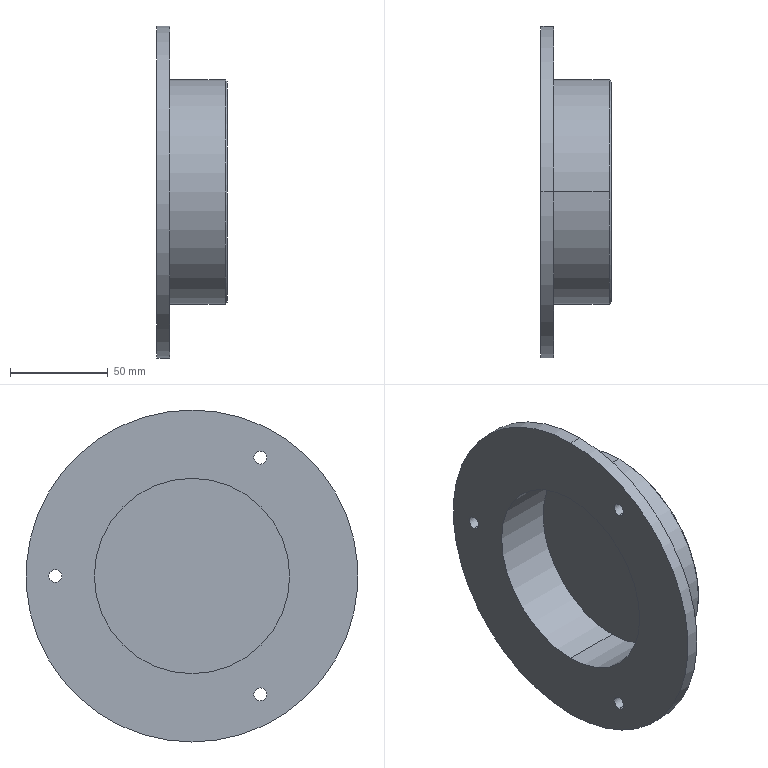Part | SolidWorks | features Chamfer 1, HoleWzd 1, Revolution 1 | 1 solid | 18 faces | box 36 x 170 x 170 mm | volume 217484 mm3 | cylinder 12 | plane 4 | cone 2 | commonest cylinder face diameters 6.6 x6 100 x2 115 x2 170 x2
STEP:
#1=CARTESIAN_POINT('',(36.,0.,-56.5));
#2=VERTEX_POINT('',#1);
#3=CARTESIAN_POINT('',(36.,0.,56.5));
#4=VERTEX_POINT('',#3);
#5=CARTESIAN_POINT('',(36.,0.,0.));
#6=DIRECTION('',(1.,0.,0.));
#7=DIRECTION('',(0.,0.,1.));
#8=AXIS2_PLACEMENT_3D('',#5,#6,#7);
#9=CIRCLE('',#8,56.5);
#10=EDGE_CURVE('',#2,#4,#9,.T.);
#11=ORIENTED_EDGE('',*,*,#10,.F.);
#12=CARTESIAN_POINT('',(35.,0.,-57.5));
#13=VERTEX_POINT('',#12);
#14=CARTESIAN_POINT('',(35.,0.,-57.5));
#15=DIRECTION('',(-0.7071,0.,-0.7071));
#16=VECTOR('',#15,1000.);
#17=LINE('',#14,#16);
#18=EDGE_CURVE('',#2,#13,#17,.T.);
#19=ORIENTED_EDGE('',*,*,#18,.T.);
#20=CARTESIAN_POINT('',(35.,0.,57.5));
#21=VERTEX_POINT('',#20);
#22=CARTESIAN_POINT('',(35.,0.,0.));
#23=DIRECTION('',(-1.,0.,0.));
#24=DIRECTION('',(0.,0.,1.));
#25=AXIS2_PLACEMENT_3D('',#22,#23,#24);
#26=CIRCLE('',#25,57.5);
#27=EDGE_CURVE('',#21,#13,#26,.T.);
#28=ORIENTED_EDGE('',*,*,#27,.F.);
#29=CARTESIAN_POINT('',(35.,0.,57.5));
#30=DIRECTION('',(-0.7071,0.,0.7071));
#31=VECTOR('',#30,1000.);
#32=LINE('',#29,#31);
#33=EDGE_CURVE('',#4,#21,#32,.T.);
#34=ORIENTED_EDGE('',*,*,#33,.F.);
#35=EDGE_LOOP('',(#11,#19,#28,#34));
#36=FACE_OUTER_BOUND('',#35,.T.);
#37=CARTESIAN_POINT('',(35.,0.,0.));
#38=DIRECTION('',(-1.,0.,0.));
#39=DIRECTION('',(0.,0.,1.));
#40=AXIS2_PLACEMENT_3D('',#37,#38,#39);
#41=CONICAL_SURFACE('',#40,57.5,0.7854);
#42=ADVANCED_FACE('',(#36),#41,.T.);
#43=CARTESIAN_POINT('',(0.,70.,3.3));
#44=VERTEX_POINT('',#43);
#45=CARTESIAN_POINT('',(0.,70.,-3.3));
#46=VERTEX_POINT('',#45);
#47=CARTESIAN_POINT('',(0.,70.,0.));
#48=DIRECTION('',(1.,0.,0.));
#49=DIRECTION('',(0.,0.,-1.));
#50=AXIS2_PLACEMENT_3D('',#47,#48,#49);
#51=CIRCLE('',#50,3.3);
#52=EDGE_CURVE('',#44,#46,#51,.T.);
#53=ORIENTED_EDGE('',*,*,#52,.F.);
#54=CARTESIAN_POINT('',(6.5,70.,3.3));
#55=VERTEX_POINT('',#54);
#56=CARTESIAN_POINT('',(6.5,70.,3.3));
#57=DIRECTION('',(1.,0.,0.));
#58=VECTOR('',#57,1000.);
#59=LINE('',#56,#58);
#60=EDGE_CURVE('',#44,#55,#59,.T.);
#61=ORIENTED_EDGE('',*,*,#60,.T.);
#62=CARTESIAN_POINT('',(6.5,70.,-3.3));
#63=VERTEX_POINT('',#62);
#64=CARTESIAN_POINT('',(6.5,70.,0.));
#65=DIRECTION('',(1.,0.,0.));
#66=DIRECTION('',(0.,0.,-1.));
#67=AXIS2_PLACEMENT_3D('',#64,#65,#66);
#68=CIRCLE('',#67,3.3);
#69=EDGE_CURVE('',#55,#63,#68,.T.);
#70=ORIENTED_EDGE('',*,*,#69,.T.);
#71=CARTESIAN_POINT('',(6.5,70.,-3.3));
#72=DIRECTION('',(1.,0.,0.));
#73=VECTOR('',#72,1000.);
#74=LINE('',#71,#73);
#75=EDGE_CURVE('',#46,#63,#74,.T.);
#76=ORIENTED_EDGE('',*,*,#75,.F.);
#77=EDGE_LOOP('',(#53,#61,#70,#76));
#78=FACE_OUTER_BOUND('',#77,.T.);
#79=CARTESIAN_POINT('',(6.5,70.,0.));
#80=DIRECTION('',(1.,0.,0.));
#81=DIRECTION('',(0.,0.,-1.));
#82=AXIS2_PLACEMENT_3D('',#79,#80,#81);
#83=CYLINDRICAL_SURFACE('',#82,3.3);
#84=ADVANCED_FACE('',(#78),#83,.F.);
#85=CARTESIAN_POINT('',(0.,-35.,-57.322));
#86=VERTEX_POINT('',#85);
#87=CARTESIAN_POINT('',(0.,-35.,-63.922));
#88=VERTEX_POINT('',#87);
#89=CARTESIAN_POINT('',(0.,-35.,-60.622));
#90=DIRECTION('',(1.,0.,0.));
#91=DIRECTION('',(0.,0.,-1.));
#92=AXIS2_PLACEMENT_3D('',#89,#90,#91);
#93=CIRCLE('',#92,3.3);
#94=EDGE_CURVE('',#86,#88,#93,.T.);
#95=ORIENTED_EDGE('',*,*,#94,.F.);
#96=CARTESIAN_POINT('',(6.5,-35.,-57.322));
#97=VERTEX_POINT('',#96);
#98=CARTESIAN_POINT('',(6.5,-35.,-57.322));
#99=DIRECTION('',(1.,0.,0.));
#100=VECTOR('',#99,1000.);
#101=LINE('',#98,#100);
#102=EDGE_CURVE('',#86,#97,#101,.T.);
#103=ORIENTED_EDGE('',*,*,#102,.T.);
#104=CARTESIAN_POINT('',(6.5,-35.,-63.922));
#105=VERTEX_POINT('',#104);
#106=CARTESIAN_POINT('',(6.5,-35.,-60.622));
#107=DIRECTION('',(1.,0.,0.));
#108=DIRECTION('',(0.,0.,-1.));
#109=AXIS2_PLACEMENT_3D('',#106,#107,#108);
#110=CIRCLE('',#109,3.3);
#111=EDGE_CURVE('',#97,#105,#110,.T.);
#112=ORIENTED_EDGE('',*,*,#111,.T.);
#113=CARTESIAN_POINT('',(6.5,-35.,-63.922));
#114=DIRECTION('',(1.,0.,0.));
#115=VECTOR('',#114,1000.);
#116=LINE('',#113,#115);
#117=EDGE_CURVE('',#88,#105,#116,.T.);
#118=ORIENTED_EDGE('',*,*,#117,.F.);
#119=EDGE_LOOP('',(#95,#103,#112,#118));
#120=FACE_OUTER_BOUND('',#119,.T.);
#121=CARTESIAN_POINT('',(6.5,-35.,-60.622));
#122=DIRECTION('',(1.,0.,0.));
#123=DIRECTION('',(0.,0.,-1.));
#124=AXIS2_PLACEMENT_3D('',#121,#122,#123);
#125=CYLINDRICAL_SURFACE('',#124,3.3);
#126=ADVANCED_FACE('',(#120),#125,.F.);
#127=CARTESIAN_POINT('',(0.,-35.,63.922));
#128=VERTEX_POINT('',#127);
#129=CARTESIAN_POINT('',(0.,-35.,57.322));
#130=VERTEX_POINT('',#129);
#131=CARTESIAN_POINT('',(0.,-35.,60.622));
#132=DIRECTION('',(1.,0.,0.));
#133=DIRECTION('',(0.,0.,-1.));
#134=AXIS2_PLACEMENT_3D('',#131,#132,#133);
#135=CIRCLE('',#134,3.3);
#136=EDGE_CURVE('',#128,#130,#135,.T.);
#137=ORIENTED_EDGE('',*,*,#136,.F.);
#138=CARTESIAN_POINT('',(6.5,-35.,63.922));
#139=VERTEX_POINT('',#138);
#140=CARTESIAN_POINT('',(6.5,-35.,63.922));
#141=DIRECTION('',(1.,0.,0.));
#142=VECTOR('',#141,1000.);
#143=LINE('',#140,#142);
#144=EDGE_CURVE('',#128,#139,#143,.T.);
#145=ORIENTED_EDGE('',*,*,#144,.T.);
#146=CARTESIAN_POINT('',(6.5,-35.,57.322));
#147=VERTEX_POINT('',#146);
#148=CARTESIAN_POINT('',(6.5,-35.,60.622));
#149=DIRECTION('',(1.,0.,0.));
#150=DIRECTION('',(0.,0.,-1.));
#151=AXIS2_PLACEMENT_3D('',#148,#149,#150);
#152=CIRCLE('',#151,3.3);
#153=EDGE_CURVE('',#139,#147,#152,.T.);
#154=ORIENTED_EDGE('',*,*,#153,.T.);
#155=CARTESIAN_POINT('',(6.5,-35.,57.322));
#156=DIRECTION('',(1.,0.,0.));
#157=VECTOR('',#156,1000.);
#158=LINE('',#155,#157);
#159=EDGE_CURVE('',#130,#147,#158,.T.);
#160=ORIENTED_EDGE('',*,*,#159,.F.);
#161=EDGE_LOOP('',(#137,#145,#154,#160));
#162=FACE_OUTER_BOUND('',#161,.T.);
#163=CARTESIAN_POINT('',(6.5,-35.,60.622));
#164=DIRECTION('',(1.,0.,0.));
#165=DIRECTION('',(0.,0.,-1.));
#166=AXIS2_PLACEMENT_3D('',#163,#164,#165);
#167=CYLINDRICAL_SURFACE('',#166,3.3);
#168=ADVANCED_FACE('',(#162),#167,.F.);
#169=ORIENTED_EDGE('',*,*,#27,.T.);
#170=CARTESIAN_POINT('',(6.5,0.,-57.5));
#171=VERTEX_POINT('',#170);
#172=CARTESIAN_POINT('',(0.,0.,-57.5));
#173=DIRECTION('',(-1.,0.,0.));
#174=VECTOR('',#173,1000.);
#175=LINE('',#172,#174);
#176=EDGE_CURVE('',#13,#171,#175,.T.);
#177=ORIENTED_EDGE('',*,*,#176,.T.);
#178=CARTESIAN_POINT('',(6.5,0.,57.5));
#179=VERTEX_POINT('',#178);
#180=CARTESIAN_POINT('',(6.5,0.,0.));
#181=DIRECTION('',(-1.,0.,0.));
#182=DIRECTION('',(0.,0.,1.));
#183=AXIS2_PLACEMENT_3D('',#180,#181,#182);
#184=CIRCLE('',#183,57.5);
#185=EDGE_CURVE('',#179,#171,#184,.T.);
#186=ORIENTED_EDGE('',*,*,#185,.F.);
#187=CARTESIAN_POINT('',(0.,0.,57.5));
#188=DIRECTION('',(-1.,0.,0.));
#189=VECTOR('',#188,1000.);
#190=LINE('',#187,#189);
#191=EDGE_CURVE('',#21,#179,#190,.T.);
#192=ORIENTED_EDGE('',*,*,#191,.F.);
#193=EDGE_LOOP('',(#169,#177,#186,#192));
#194=FACE_OUTER_BOUND('',#193,.T.);
#195=CARTESIAN_POINT('',(0.,0.,0.));
#196=DIRECTION('',(-1.,0.,0.));
#197=DIRECTION('',(0.,0.,1.));
#198=AXIS2_PLACEMENT_3D('',#195,#196,#197);
#199=CYLINDRICAL_SURFACE('',#198,57.5);
#200=ADVANCED_FACE('',(#194),#199,.T.);
#201=CARTESIAN_POINT('',(6.5,0.,85.));
#202=VERTEX_POINT('',#201);
#203=CARTESIAN_POINT('',(6.5,0.,-85.));
#204=VERTEX_POINT('',#203);
#205=CARTESIAN_POINT('',(6.5,0.,0.));
#206=DIRECTION('',(-1.,0.,0.));
#207=DIRECTION('',(0.,0.,1.));
#208=AXIS2_PLACEMENT_3D('',#205,#206,#207);
#209=CIRCLE('',#208,85.);
#210=EDGE_CURVE('',#202,#204,#209,.T.);
#211=ORIENTED_EDGE('',*,*,#210,.T.);
#212=CARTESIAN_POINT('',(0.,0.,-85.));
#213=VERTEX_POINT('',#212);
#214=CARTESIAN_POINT('',(0.,0.,-85.));
#215=DIRECTION('',(-1.,0.,0.));
#216=VECTOR('',#215,1000.);
#217=LINE('',#214,#216);
#218=EDGE_CURVE('',#204,#213,#217,.T.);
#219=ORIENTED_EDGE('',*,*,#218,.T.);
#220=CARTESIAN_POINT('',(0.,0.,85.));
#221=VERTEX_POINT('',#220);
#222=CARTESIAN_POINT('',(0.,0.,0.));
#223=DIRECTION('',(-1.,0.,0.));
#224=DIRECTION('',(0.,0.,1.));
#225=AXIS2_PLACEMENT_3D('',#222,#223,#224);
#226=CIRCLE('',#225,85.);
#227=EDGE_CURVE('',#221,#213,#226,.T.);
#228=ORIENTED_EDGE('',*,*,#227,.F.);
#229=CARTESIAN_POINT('',(0.,0.,85.));
#230=DIRECTION('',(-1.,0.,0.));
#231=VECTOR('',#230,1000.);
#232=LINE('',#229,#231);
#233=EDGE_CURVE('',#202,#221,#232,.T.);
#234=ORIENTED_EDGE('',*,*,#233,.F.);
#235=EDGE_LOOP('',(#211,#219,#228,#234));
#236=FACE_OUTER_BOUND('',#235,.T.);
#237=CARTESIAN_POINT('',(0.,0.,0.));
#238=DIRECTION('',(-1.,0.,0.));
#239=DIRECTION('',(0.,0.,1.));
#240=AXIS2_PLACEMENT_3D('',#237,#238,#239);
#241=CYLINDRICAL_SURFACE('',#240,85.);
#242=ADVANCED_FACE('',(#236),#241,.T.);
#243=CARTESIAN_POINT('',(30.,0.,-50.));
#244=VERTEX_POINT('',#243);
#245=CARTESIAN_POINT('',(30.,0.,50.));
#246=VERTEX_POINT('',#245);
#247=CARTESIAN_POINT('',(30.,0.,0.));
#248=DIRECTION('',(-1.,0.,0.));
#249=DIRECTION('',(0.,0.,1.));
#250=AXIS2_PLACEMENT_3D('',#247,#248,#249);
#251=CIRCLE('',#250,50.);
#252=EDGE_CURVE('',#244,#246,#251,.T.);
#253=ORIENTED_EDGE('',*,*,#252,.F.);
#254=CARTESIAN_POINT('',(0.,0.,-50.));
#255=VERTEX_POINT('',#254);
#256=CARTESIAN_POINT('',(0.,0.,-50.));
#257=DIRECTION('',(-1.,0.,0.));
#258=VECTOR('',#257,1000.);
#259=LINE('',#256,#258);
#260=EDGE_CURVE('',#244,#255,#259,.T.);
#261=ORIENTED_EDGE('',*,*,#260,.T.);
#262=CARTESIAN_POINT('',(0.,0.,50.));
#263=VERTEX_POINT('',#262);
#264=CARTESIAN_POINT('',(0.,0.,0.));
#265=DIRECTION('',(-1.,0.,0.));
#266=DIRECTION('',(0.,0.,1.));
#267=AXIS2_PLACEMENT_3D('',#264,#265,#266);
#268=CIRCLE('',#267,50.);
#269=EDGE_CURVE('',#255,#263,#268,.T.);
#270=ORIENTED_EDGE('',*,*,#269,.T.);
#271=CARTESIAN_POINT('',(0.,0.,50.));
#272=DIRECTION('',(-1.,0.,0.));
#273=VECTOR('',#272,1000.);
#274=LINE('',#271,#273);
#275=EDGE_CURVE('',#246,#263,#274,.T.);
#276=ORIENTED_EDGE('',*,*,#275,.F.);
#277=EDGE_LOOP('',(#253,#261,#270,#276));
#278=FACE_OUTER_BOUND('',#277,.T.);
#279=CARTESIAN_POINT('',(0.,0.,0.));
#280=DIRECTION('',(-1.,0.,0.));
#281=DIRECTION('',(0.,0.,1.));
#282=AXIS2_PLACEMENT_3D('',#279,#280,#281);
#283=CYLINDRICAL_SURFACE('',#282,50.);
#284=ADVANCED_FACE('',(#278),#283,.F.);
#285=CARTESIAN_POINT('',(6.5,70.,0.));
#286=DIRECTION('',(1.,0.,0.));
#287=DIRECTION('',(0.,0.,-1.));
#288=AXIS2_PLACEMENT_3D('',#285,#286,#287);
#289=CIRCLE('',#288,3.3);
#290=EDGE_CURVE('',#63,#55,#289,.T.);
#291=ORIENTED_EDGE('',*,*,#290,.F.);
#292=ORIENTED_EDGE('',*,*,#69,.F.);
#293=EDGE_LOOP('',(#291,#292));
#294=FACE_BOUND('',#293,.T.);
#295=ORIENTED_EDGE('',*,*,#210,.F.);
#296=CARTESIAN_POINT('',(6.5,0.,0.));
#297=DIRECTION('',(-1.,0.,0.));
#298=DIRECTION('',(0.,0.,1.));
#299=AXIS2_PLACEMENT_3D('',#296,#297,#298);
#300=CIRCLE('',#299,85.);
#301=EDGE_CURVE('',#204,#202,#300,.T.);
#302=ORIENTED_EDGE('',*,*,#301,.F.);
#303=EDGE_LOOP('',(#295,#302));
#304=FACE_OUTER_BOUND('',#303,.T.);
#305=ORIENTED_EDGE('',*,*,#185,.T.);
#306=CARTESIAN_POINT('',(6.5,0.,0.));
#307=DIRECTION('',(-1.,0.,0.));
#308=DIRECTION('',(0.,0.,1.));
#309=AXIS2_PLACEMENT_3D('',#306,#307,#308);
#310=CIRCLE('',#309,57.5);
#311=EDGE_CURVE('',#171,#179,#310,.T.);
#312=ORIENTED_EDGE('',*,*,#311,.T.);
#313=EDGE_LOOP('',(#305,#312));
#314=FACE_BOUND('',#313,.T.);
#315=CARTESIAN_POINT('',(6.5,-35.,60.622));
#316=DIRECTION('',(1.,0.,0.));
#317=DIRECTION('',(0.,0.,-1.));
#318=AXIS2_PLACEMENT_3D('',#315,#316,#317);
#319=CIRCLE('',#318,3.3);
#320=EDGE_CURVE('',#147,#139,#319,.T.);
#321=ORIENTED_EDGE('',*,*,#320,.F.);
#322=ORIENTED_EDGE('',*,*,#153,.F.);
#323=EDGE_LOOP('',(#321,#322));
#324=FACE_BOUND('',#323,.T.);
#325=CARTESIAN_POINT('',(6.5,-35.,-60.622));
#326=DIRECTION('',(1.,0.,0.));
#327=DIRECTION('',(0.,0.,-1.));
#328=AXIS2_PLACEMENT_3D('',#325,#326,#327);
#329=CIRCLE('',#328,3.3);
#330=EDGE_CURVE('',#105,#97,#329,.T.);
#331=ORIENTED_EDGE('',*,*,#330,.F.);
#332=ORIENTED_EDGE('',*,*,#111,.F.);
#333=EDGE_LOOP('',(#331,#332));
#334=FACE_BOUND('',#333,.T.);
#335=CARTESIAN_POINT('',(6.5,85.,0.));
#336=DIRECTION('',(-1.,0.,0.));
#337=DIRECTION('',(0.,0.,1.));
#338=AXIS2_PLACEMENT_3D('',#335,#336,#337);
#339=PLANE('',#338);
#340=ADVANCED_FACE('',(#294,#304,#314,#324,#334),#339,.F.);
#341=CARTESIAN_POINT('',(30.,0.,0.));
#342=DIRECTION('',(-1.,0.,0.));
#343=DIRECTION('',(0.,0.,1.));
#344=AXIS2_PLACEMENT_3D('',#341,#342,#343);
#345=CIRCLE('',#344,50.);
#346=EDGE_CURVE('',#246,#244,#345,.T.);
#347=ORIENTED_EDGE('',*,*,#346,.T.);
#348=ORIENTED_EDGE('',*,*,#252,.T.);
#349=EDGE_LOOP('',(#347,#348));
#350=FACE_OUTER_BOUND('',#349,.T.);
#351=CARTESIAN_POINT('',(30.,0.,0.));
#352=DIRECTION('',(1.,0.,0.));
#353=DIRECTION('',(0.,0.,-1.));
#354=AXIS2_PLACEMENT_3D('',#351,#352,#353);
#355=PLANE('',#354);
#356=ADVANCED_FACE('',(#350),#355,.F.);
#357=ORIENTED_EDGE('',*,*,#260,.F.);
#358=ORIENTED_EDGE('',*,*,#346,.F.);
#359=ORIENTED_EDGE('',*,*,#275,.T.);
#360=CARTESIAN_POINT('',(0.,0.,0.));
#361=DIRECTION('',(-1.,0.,0.));
#362=DIRECTION('',(0.,0.,1.));
#363=AXIS2_PLACEMENT_3D('',#360,#361,#362);
#364=CIRCLE('',#363,50.);
#365=EDGE_CURVE('',#263,#255,#364,.T.);
#366=ORIENTED_EDGE('',*,*,#365,.T.);
#367=EDGE_LOOP('',(#357,#358,#359,#366));
#368=FACE_OUTER_BOUND('',#367,.T.);
#369=CARTESIAN_POINT('',(0.,0.,0.));
#370=DIRECTION('',(-1.,0.,0.));
#371=DIRECTION('',(0.,0.,1.));
#372=AXIS2_PLACEMENT_3D('',#369,#370,#371);
#373=CYLINDRICAL_SURFACE('',#372,50.);
#374=ADVANCED_FACE('',(#368),#373,.F.);
#375=CARTESIAN_POINT('',(0.,70.,0.));
#376=DIRECTION('',(1.,0.,0.));
#377=DIRECTION('',(0.,0.,-1.));
#378=AXIS2_PLACEMENT_3D('',#375,#376,#377);
#379=CIRCLE('',#378,3.3);
#380=EDGE_CURVE('',#46,#44,#379,.T.);
#381=ORIENTED_EDGE('',*,*,#380,.T.);
#382=ORIENTED_EDGE('',*,*,#52,.T.);
#383=EDGE_LOOP('',(#381,#382));
#384=FACE_BOUND('',#383,.T.);
#385=CARTESIAN_POINT('',(0.,-35.,-60.622));
#386=DIRECTION('',(1.,0.,0.));
#387=DIRECTION('',(0.,0.,-1.));
#388=AXIS2_PLACEMENT_3D('',#385,#386,#387);
#389=CIRCLE('',#388,3.3);
#390=EDGE_CURVE('',#88,#86,#389,.T.);
#391=ORIENTED_EDGE('',*,*,#390,.T.);
#392=ORIENTED_EDGE('',*,*,#94,.T.);
#393=EDGE_LOOP('',(#391,#392));
#394=FACE_BOUND('',#393,.T.);
#395=CARTESIAN_POINT('',(0.,-35.,60.622));
#396=DIRECTION('',(1.,0.,0.));
#397=DIRECTION('',(0.,0.,-1.));
#398=AXIS2_PLACEMENT_3D('',#395,#396,#397);
#399=CIRCLE('',#398,3.3);
#400=EDGE_CURVE('',#130,#128,#399,.T.);
#401=ORIENTED_EDGE('',*,*,#400,.T.);
#402=ORIENTED_EDGE('',*,*,#136,.T.);
#403=EDGE_LOOP('',(#401,#402));
#404=FACE_BOUND('',#403,.T.);
#405=ORIENTED_EDGE('',*,*,#365,.F.);
#406=ORIENTED_EDGE('',*,*,#269,.F.);
#407=EDGE_LOOP('',(#405,#406));
#408=FACE_BOUND('',#407,.T.);
#409=ORIENTED_EDGE('',*,*,#227,.T.);
#410=CARTESIAN_POINT('',(0.,0.,0.));
#411=DIRECTION('',(-1.,0.,0.));
#412=DIRECTION('',(0.,0.,1.));
#413=AXIS2_PLACEMENT_3D('',#410,#411,#412);
#414=CIRCLE('',#413,85.);
#415=EDGE_CURVE('',#213,#221,#414,.T.);
#416=ORIENTED_EDGE('',*,*,#415,.T.);
#417=EDGE_LOOP('',(#409,#416));
#418=FACE_OUTER_BOUND('',#417,.T.);
#419=CARTESIAN_POINT('',(0.,50.,0.));
#420=DIRECTION('',(1.,0.,0.));
#421=DIRECTION('',(0.,0.,-1.));
#422=AXIS2_PLACEMENT_3D('',#419,#420,#421);
#423=PLANE('',#422);
#424=ADVANCED_FACE('',(#384,#394,#404,#408,#418),#423,.F.);
#425=ORIENTED_EDGE('',*,*,#218,.F.);
#426=ORIENTED_EDGE('',*,*,#301,.T.);
#427=ORIENTED_EDGE('',*,*,#233,.T.);
#428=ORIENTED_EDGE('',*,*,#415,.F.);
#429=EDGE_LOOP('',(#425,#426,#427,#428));
#430=FACE_OUTER_BOUND('',#429,.T.);
#431=CARTESIAN_POINT('',(0.,0.,0.));
#432=DIRECTION('',(-1.,0.,0.));
#433=DIRECTION('',(0.,0.,1.));
#434=AXIS2_PLACEMENT_3D('',#431,#432,#433);
#435=CYLINDRICAL_SURFACE('',#434,85.);
#436=ADVANCED_FACE('',(#430),#435,.T.);
#437=ORIENTED_EDGE('',*,*,#176,.F.);
#438=CARTESIAN_POINT('',(35.,0.,0.));
#439=DIRECTION('',(-1.,0.,0.));
#440=DIRECTION('',(0.,0.,1.));
#441=AXIS2_PLACEMENT_3D('',#438,#439,#440);
#442=CIRCLE('',#441,57.5);
#443=EDGE_CURVE('',#13,#21,#442,.T.);
#444=ORIENTED_EDGE('',*,*,#443,.T.);
#445=ORIENTED_EDGE('',*,*,#191,.T.);
#446=ORIENTED_EDGE('',*,*,#311,.F.);
#447=EDGE_LOOP('',(#437,#444,#445,#446));
#448=FACE_OUTER_BOUND('',#447,.T.);
#449=CARTESIAN_POINT('',(0.,0.,0.));
#450=DIRECTION('',(-1.,0.,0.));
#451=DIRECTION('',(0.,0.,1.));
#452=AXIS2_PLACEMENT_3D('',#449,#450,#451);
#453=CYLINDRICAL_SURFACE('',#452,57.5);
#454=ADVANCED_FACE('',(#448),#453,.T.);
#455=CARTESIAN_POINT('',(36.,0.,0.));
#456=DIRECTION('',(1.,0.,0.));
#457=DIRECTION('',(0.,0.,1.));
#458=AXIS2_PLACEMENT_3D('',#455,#456,#457);
#459=CIRCLE('',#458,56.5);
#460=EDGE_CURVE('',#4,#2,#459,.T.);
#461=ORIENTED_EDGE('',*,*,#460,.T.);
#462=ORIENTED_EDGE('',*,*,#10,.T.);
#463=EDGE_LOOP('',(#461,#462));
#464=FACE_OUTER_BOUND('',#463,.T.);
#465=CARTESIAN_POINT('',(36.,57.5,0.));
#466=DIRECTION('',(-1.,0.,0.));
#467=DIRECTION('',(0.,0.,1.));
#468=AXIS2_PLACEMENT_3D('',#465,#466,#467);
#469=PLANE('',#468);
#470=ADVANCED_FACE('',(#464),#469,.F.);
#471=ORIENTED_EDGE('',*,*,#144,.F.);
#472=ORIENTED_EDGE('',*,*,#400,.F.);
#473=ORIENTED_EDGE('',*,*,#159,.T.);
#474=ORIENTED_EDGE('',*,*,#320,.T.);
#475=EDGE_LOOP('',(#471,#472,#473,#474));
#476=FACE_OUTER_BOUND('',#475,.T.);
#477=CARTESIAN_POINT('',(6.5,-35.,60.622));
#478=DIRECTION('',(1.,0.,0.));
#479=DIRECTION('',(0.,0.,-1.));
#480=AXIS2_PLACEMENT_3D('',#477,#478,#479);
#481=CYLINDRICAL_SURFACE('',#480,3.3);
#482=ADVANCED_FACE('',(#476),#481,.F.);
#483=ORIENTED_EDGE('',*,*,#102,.F.);
#484=ORIENTED_EDGE('',*,*,#390,.F.);
#485=ORIENTED_EDGE('',*,*,#117,.T.);
#486=ORIENTED_EDGE('',*,*,#330,.T.);
#487=EDGE_LOOP('',(#483,#484,#485,#486));
#488=FACE_OUTER_BOUND('',#487,.T.);
#489=CARTESIAN_POINT('',(6.5,-35.,-60.622));
#490=DIRECTION('',(1.,0.,0.));
#491=DIRECTION('',(0.,0.,-1.));
#492=AXIS2_PLACEMENT_3D('',#489,#490,#491);
#493=CYLINDRICAL_SURFACE('',#492,3.3);
#494=ADVANCED_FACE('',(#488),#493,.F.);
#495=ORIENTED_EDGE('',*,*,#60,.F.);
#496=ORIENTED_EDGE('',*,*,#380,.F.);
#497=ORIENTED_EDGE('',*,*,#75,.T.);
#498=ORIENTED_EDGE('',*,*,#290,.T.);
#499=EDGE_LOOP('',(#495,#496,#497,#498));
#500=FACE_OUTER_BOUND('',#499,.T.);
#501=CARTESIAN_POINT('',(6.5,70.,0.));
#502=DIRECTION('',(1.,0.,0.));
#503=DIRECTION('',(0.,0.,-1.));
#504=AXIS2_PLACEMENT_3D('',#501,#502,#503);
#505=CYLINDRICAL_SURFACE('',#504,3.3);
#506=ADVANCED_FACE('',(#500),#505,.F.);
#507=ORIENTED_EDGE('',*,*,#18,.F.);
#508=ORIENTED_EDGE('',*,*,#460,.F.);
#509=ORIENTED_EDGE('',*,*,#33,.T.);
#510=ORIENTED_EDGE('',*,*,#443,.F.);
#511=EDGE_LOOP('',(#507,#508,#509,#510));
#512=FACE_OUTER_BOUND('',#511,.T.);
#513=CARTESIAN_POINT('',(35.,0.,0.));
#514=DIRECTION('',(-1.,0.,0.));
#515=DIRECTION('',(0.,0.,1.));
#516=AXIS2_PLACEMENT_3D('',#513,#514,#515);
#517=CONICAL_SURFACE('',#516,57.5,0.7854);
#518=ADVANCED_FACE('',(#512),#517,.T.);
#519=CLOSED_SHELL('',(#42,#84,#126,#168,#200,#242,#284,#340,#356,#374,#424,#436,#454,#470,#482,#494,#506,#518));
#520=MANIFOLD_SOLID_BREP('',#519);
#521=CARTESIAN_POINT('',(0.,0.,0.));
#522=DIRECTION('',(0.,0.,1.));
#523=DIRECTION('',(1.,0.,0.));
#524=AXIS2_PLACEMENT_3D('',#521,#522,#523);
#525=(LENGTH_UNIT()NAMED_UNIT(*)SI_UNIT(.MILLI.,.METRE.));
#526=UNCERTAINTY_MEASURE_WITH_UNIT(LENGTH_MEASURE(0.00001),#525,'','');
#527=(NAMED_UNIT(*)PLANE_ANGLE_UNIT()SI_UNIT($,.RADIAN.));
#528=(NAMED_UNIT(*)SI_UNIT($,.STERADIAN.)SOLID_ANGLE_UNIT());
#529=(GEOMETRIC_REPRESENTATION_CONTEXT(3)GLOBAL_UNCERTAINTY_ASSIGNED_CONTEXT((#526))GLOBAL_UNIT_ASSIGNED_CONTEXT((#525,#527,#528))REPRESENTATION_CONTEXT('',''));
#530=ADVANCED_BREP_SHAPE_REPRESENTATION('',(#520,#524),#529);